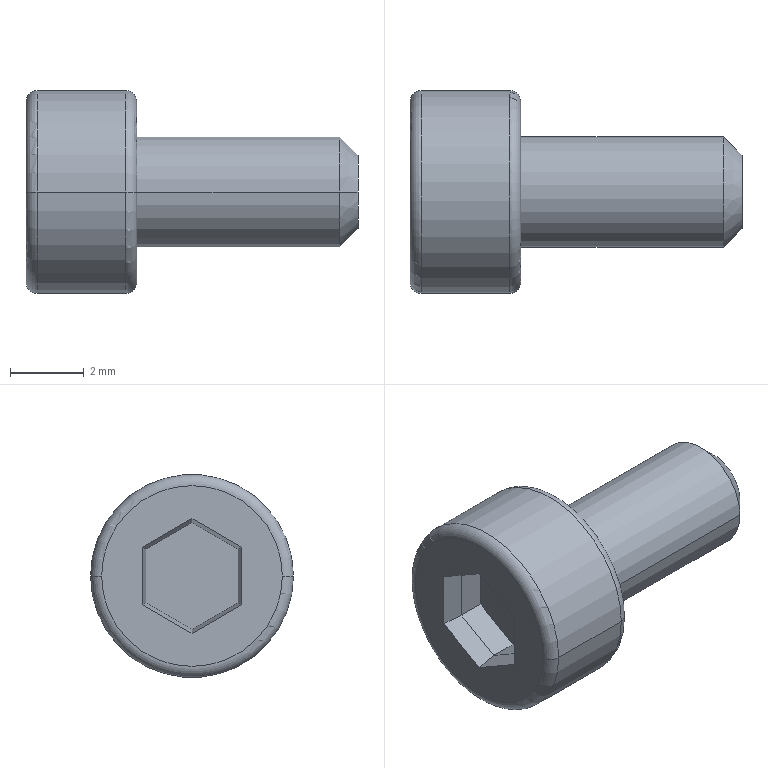Part | SolidWorks | features Chamfer 2, Fillet 1, ICE 1, Revolution 1 | 1 solid | 26 faces | box 9 x 5.5 x 5.5 mm | volume 104.699 mm3 | plane 16 | torus 4 | cylinder 4 | cone 2 | commonest cylinder face diameters 3 x2 5.5 x2
STEP:
#1=CARTESIAN_POINT('',(9.,1.,0.));
#2=VERTEX_POINT('',#1);
#3=CARTESIAN_POINT('',(9.,-1.,0.));
#4=VERTEX_POINT('',#3);
#5=CARTESIAN_POINT('',(9.,0.,0.));
#6=DIRECTION('',(1.,0.,0.));
#7=DIRECTION('',(0.,-1.,0.));
#8=AXIS2_PLACEMENT_3D('',#5,#6,#7);
#9=CIRCLE('',#8,1.);
#10=EDGE_CURVE('',#2,#4,#9,.T.);
#11=ORIENTED_EDGE('',*,*,#10,.F.);
#12=CARTESIAN_POINT('',(8.5,1.5,0.));
#13=VERTEX_POINT('',#12);
#14=CARTESIAN_POINT('',(8.5,1.5,0.));
#15=DIRECTION('',(-0.7071,0.7071,0.));
#16=VECTOR('',#15,1000.);
#17=LINE('',#14,#16);
#18=EDGE_CURVE('',#2,#13,#17,.T.);
#19=ORIENTED_EDGE('',*,*,#18,.T.);
#20=CARTESIAN_POINT('',(8.5,-1.5,0.));
#21=VERTEX_POINT('',#20);
#22=CARTESIAN_POINT('',(8.5,0.,0.));
#23=DIRECTION('',(-1.,0.,0.));
#24=DIRECTION('',(0.,-1.,0.));
#25=AXIS2_PLACEMENT_3D('',#22,#23,#24);
#26=CIRCLE('',#25,1.5);
#27=EDGE_CURVE('',#21,#13,#26,.T.);
#28=ORIENTED_EDGE('',*,*,#27,.F.);
#29=CARTESIAN_POINT('',(8.5,-1.5,0.));
#30=DIRECTION('',(-0.7071,-0.7071,0.));
#31=VECTOR('',#30,1000.);
#32=LINE('',#29,#31);
#33=EDGE_CURVE('',#4,#21,#32,.T.);
#34=ORIENTED_EDGE('',*,*,#33,.F.);
#35=EDGE_LOOP('',(#11,#19,#28,#34));
#36=FACE_OUTER_BOUND('',#35,.T.);
#37=CARTESIAN_POINT('',(8.5,0.,0.));
#38=DIRECTION('',(-1.,0.,0.));
#39=DIRECTION('',(0.,-1.,0.));
#40=AXIS2_PLACEMENT_3D('',#37,#38,#39);
#41=CONICAL_SURFACE('',#40,1.5,0.7854);
#42=ADVANCED_FACE('',(#36),#41,.T.);
#43=CARTESIAN_POINT('',(0.,-2.45,0.));
#44=VERTEX_POINT('',#43);
#45=CARTESIAN_POINT('',(0.,2.45,0.));
#46=VERTEX_POINT('',#45);
#47=CARTESIAN_POINT('',(0.,0.,0.));
#48=DIRECTION('',(-1.,0.,0.));
#49=DIRECTION('',(0.,1.,0.));
#50=AXIS2_PLACEMENT_3D('',#47,#48,#49);
#51=CIRCLE('',#50,2.45);
#52=EDGE_CURVE('',#44,#46,#51,.T.);
#53=ORIENTED_EDGE('',*,*,#52,.F.);
#54=CARTESIAN_POINT('',(0.3,-2.75,0.));
#55=VERTEX_POINT('',#54);
#56=CARTESIAN_POINT('',(0.3,-2.45,0.));
#57=DIRECTION('',(0.,0.,1.));
#58=DIRECTION('',(0.,-1.,0.));
#59=AXIS2_PLACEMENT_3D('',#56,#57,#58);
#60=CIRCLE('',#59,0.3);
#61=EDGE_CURVE('',#44,#55,#60,.T.);
#62=ORIENTED_EDGE('',*,*,#61,.T.);
#63=CARTESIAN_POINT('',(0.3,2.75,0.));
#64=VERTEX_POINT('',#63);
#65=CARTESIAN_POINT('',(0.3,0.,0.));
#66=DIRECTION('',(1.,0.,0.));
#67=DIRECTION('',(0.,1.,0.));
#68=AXIS2_PLACEMENT_3D('',#65,#66,#67);
#69=CIRCLE('',#68,2.75);
#70=EDGE_CURVE('',#64,#55,#69,.T.);
#71=ORIENTED_EDGE('',*,*,#70,.F.);
#72=CARTESIAN_POINT('',(0.3,2.45,0.));
#73=DIRECTION('',(0.,0.,-1.));
#74=DIRECTION('',(-1.,0.,0.));
#75=AXIS2_PLACEMENT_3D('',#72,#73,#74);
#76=CIRCLE('',#75,0.3);
#77=EDGE_CURVE('',#46,#64,#76,.T.);
#78=ORIENTED_EDGE('',*,*,#77,.F.);
#79=EDGE_LOOP('',(#53,#62,#71,#78));
#80=FACE_OUTER_BOUND('',#79,.T.);
#81=CARTESIAN_POINT('',(0.3,0.,0.));
#82=DIRECTION('',(1.,0.,0.));
#83=DIRECTION('',(0.,1.,0.));
#84=AXIS2_PLACEMENT_3D('',#81,#82,#83);
#85=TOROIDAL_SURFACE('',#84,2.45,0.3);
#86=ADVANCED_FACE('',(#80),#85,.T.);
#87=CARTESIAN_POINT('',(3.,2.45,0.));
#88=VERTEX_POINT('',#87);
#89=CARTESIAN_POINT('',(3.,-2.45,0.));
#90=VERTEX_POINT('',#89);
#91=CARTESIAN_POINT('',(3.,0.,0.));
#92=DIRECTION('',(1.,0.,0.));
#93=DIRECTION('',(0.,-1.,0.));
#94=AXIS2_PLACEMENT_3D('',#91,#92,#93);
#95=CIRCLE('',#94,2.45);
#96=EDGE_CURVE('',#88,#90,#95,.T.);
#97=ORIENTED_EDGE('',*,*,#96,.F.);
#98=CARTESIAN_POINT('',(2.7,2.75,0.));
#99=VERTEX_POINT('',#98);
#100=CARTESIAN_POINT('',(2.7,2.45,0.));
#101=DIRECTION('',(0.,0.,1.));
#102=DIRECTION('',(0.,-1.,0.));
#103=AXIS2_PLACEMENT_3D('',#100,#101,#102);
#104=CIRCLE('',#103,0.3);
#105=EDGE_CURVE('',#88,#99,#104,.T.);
#106=ORIENTED_EDGE('',*,*,#105,.T.);
#107=CARTESIAN_POINT('',(2.7,-2.75,0.));
#108=VERTEX_POINT('',#107);
#109=CARTESIAN_POINT('',(2.7,0.,0.));
#110=DIRECTION('',(-1.,0.,0.));
#111=DIRECTION('',(0.,-1.,0.));
#112=AXIS2_PLACEMENT_3D('',#109,#110,#111);
#113=CIRCLE('',#112,2.75);
#114=EDGE_CURVE('',#108,#99,#113,.T.);
#115=ORIENTED_EDGE('',*,*,#114,.F.);
#116=CARTESIAN_POINT('',(2.7,-2.45,0.));
#117=DIRECTION('',(0.,0.,-1.));
#118=DIRECTION('',(-1.,0.,0.));
#119=AXIS2_PLACEMENT_3D('',#116,#117,#118);
#120=CIRCLE('',#119,0.3);
#121=EDGE_CURVE('',#90,#108,#120,.T.);
#122=ORIENTED_EDGE('',*,*,#121,.F.);
#123=EDGE_LOOP('',(#97,#106,#115,#122));
#124=FACE_OUTER_BOUND('',#123,.T.);
#125=CARTESIAN_POINT('',(2.7,0.,0.));
#126=DIRECTION('',(-1.,0.,0.));
#127=DIRECTION('',(0.,-1.,0.));
#128=AXIS2_PLACEMENT_3D('',#125,#126,#127);
#129=TOROIDAL_SURFACE('',#128,2.45,0.3);
#130=ADVANCED_FACE('',(#124),#129,.T.);
#131=ORIENTED_EDGE('',*,*,#27,.T.);
#132=CARTESIAN_POINT('',(3.,1.5,0.));
#133=VERTEX_POINT('',#132);
#134=CARTESIAN_POINT('',(-4.709,1.5,0.));
#135=DIRECTION('',(-1.,0.,0.));
#136=VECTOR('',#135,1000.);
#137=LINE('',#134,#136);
#138=EDGE_CURVE('',#13,#133,#137,.T.);
#139=ORIENTED_EDGE('',*,*,#138,.T.);
#140=CARTESIAN_POINT('',(3.,-1.5,0.));
#141=VERTEX_POINT('',#140);
#142=CARTESIAN_POINT('',(3.,0.,0.));
#143=DIRECTION('',(-1.,0.,0.));
#144=DIRECTION('',(0.,-1.,0.));
#145=AXIS2_PLACEMENT_3D('',#142,#143,#144);
#146=CIRCLE('',#145,1.5);
#147=EDGE_CURVE('',#141,#133,#146,.T.);
#148=ORIENTED_EDGE('',*,*,#147,.F.);
#149=CARTESIAN_POINT('',(-4.709,-1.5,0.));
#150=DIRECTION('',(-1.,0.,0.));
#151=VECTOR('',#150,1000.);
#152=LINE('',#149,#151);
#153=EDGE_CURVE('',#21,#141,#152,.T.);
#154=ORIENTED_EDGE('',*,*,#153,.F.);
#155=EDGE_LOOP('',(#131,#139,#148,#154));
#156=FACE_OUTER_BOUND('',#155,.T.);
#157=CARTESIAN_POINT('',(-4.709,0.,0.));
#158=DIRECTION('',(-1.,0.,0.));
#159=DIRECTION('',(0.,-1.,0.));
#160=AXIS2_PLACEMENT_3D('',#157,#158,#159);
#161=CYLINDRICAL_SURFACE('',#160,1.5);
#162=ADVANCED_FACE('',(#156),#161,.T.);
#163=ORIENTED_EDGE('',*,*,#114,.T.);
#164=CARTESIAN_POINT('',(-4.709,2.75,0.));
#165=DIRECTION('',(-1.,0.,0.));
#166=VECTOR('',#165,1000.);
#167=LINE('',#164,#166);
#168=EDGE_CURVE('',#99,#64,#167,.T.);
#169=ORIENTED_EDGE('',*,*,#168,.T.);
#170=ORIENTED_EDGE('',*,*,#70,.T.);
#171=CARTESIAN_POINT('',(-4.709,-2.75,0.));
#172=DIRECTION('',(-1.,0.,0.));
#173=VECTOR('',#172,1000.);
#174=LINE('',#171,#173);
#175=EDGE_CURVE('',#108,#55,#174,.T.);
#176=ORIENTED_EDGE('',*,*,#175,.F.);
#177=EDGE_LOOP('',(#163,#169,#170,#176));
#178=FACE_OUTER_BOUND('',#177,.T.);
#179=CARTESIAN_POINT('',(-4.709,0.,0.));
#180=DIRECTION('',(-1.,0.,0.));
#181=DIRECTION('',(0.,-1.,0.));
#182=AXIS2_PLACEMENT_3D('',#179,#180,#181);
#183=CYLINDRICAL_SURFACE('',#182,2.75);
#184=ADVANCED_FACE('',(#178),#183,.T.);
#185=CARTESIAN_POINT('',(0.,-1.35,0.7794));
#186=VERTEX_POINT('',#185);
#187=CARTESIAN_POINT('',(0.,-1.35,-0.7794));
#188=VERTEX_POINT('',#187);
#189=CARTESIAN_POINT('',(0.,-1.35,0.));
#190=DIRECTION('',(0.,0.,-1.));
#191=VECTOR('',#190,1000.);
#192=LINE('',#189,#191);
#193=EDGE_CURVE('',#186,#188,#192,.T.);
#194=ORIENTED_EDGE('',*,*,#193,.T.);
#195=CARTESIAN_POINT('',(0.,0.,-1.559));
#196=VERTEX_POINT('',#195);
#197=CARTESIAN_POINT('',(0.,-0.675,-1.169));
#198=DIRECTION('',(0.,0.866,-0.5));
#199=VECTOR('',#198,1000.);
#200=LINE('',#197,#199);
#201=EDGE_CURVE('',#188,#196,#200,.T.);
#202=ORIENTED_EDGE('',*,*,#201,.T.);
#203=CARTESIAN_POINT('',(0.,1.35,-0.7794));
#204=VERTEX_POINT('',#203);
#205=CARTESIAN_POINT('',(0.,0.675,-1.169));
#206=DIRECTION('',(0.,0.866,0.5));
#207=VECTOR('',#206,1000.);
#208=LINE('',#205,#207);
#209=EDGE_CURVE('',#196,#204,#208,.T.);
#210=ORIENTED_EDGE('',*,*,#209,.T.);
#211=CARTESIAN_POINT('',(0.,1.35,0.7794));
#212=VERTEX_POINT('',#211);
#213=CARTESIAN_POINT('',(0.,1.35,0.));
#214=DIRECTION('',(0.,0.,1.));
#215=VECTOR('',#214,1000.);
#216=LINE('',#213,#215);
#217=EDGE_CURVE('',#204,#212,#216,.T.);
#218=ORIENTED_EDGE('',*,*,#217,.T.);
#219=CARTESIAN_POINT('',(0.,0.,1.559));
#220=VERTEX_POINT('',#219);
#221=CARTESIAN_POINT('',(0.,0.675,1.169));
#222=DIRECTION('',(0.,-0.866,0.5));
#223=VECTOR('',#222,1000.);
#224=LINE('',#221,#223);
#225=EDGE_CURVE('',#212,#220,#224,.T.);
#226=ORIENTED_EDGE('',*,*,#225,.T.);
#227=CARTESIAN_POINT('',(0.,-0.675,1.169));
#228=DIRECTION('',(0.,-0.866,-0.5));
#229=VECTOR('',#228,1000.);
#230=LINE('',#227,#229);
#231=EDGE_CURVE('',#220,#186,#230,.T.);
#232=ORIENTED_EDGE('',*,*,#231,.T.);
#233=EDGE_LOOP('',(#194,#202,#210,#218,#226,#232));
#234=FACE_BOUND('',#233,.T.);
#235=CARTESIAN_POINT('',(0.,0.,0.));
#236=DIRECTION('',(-1.,0.,0.));
#237=DIRECTION('',(0.,1.,0.));
#238=AXIS2_PLACEMENT_3D('',#235,#236,#237);
#239=CIRCLE('',#238,2.45);
#240=EDGE_CURVE('',#46,#44,#239,.T.);
#241=ORIENTED_EDGE('',*,*,#240,.T.);
#242=ORIENTED_EDGE('',*,*,#52,.T.);
#243=EDGE_LOOP('',(#241,#242));
#244=FACE_OUTER_BOUND('',#243,.T.);
#245=CARTESIAN_POINT('',(0.,0.,0.));
#246=DIRECTION('',(1.,0.,0.));
#247=DIRECTION('',(0.,1.,0.));
#248=AXIS2_PLACEMENT_3D('',#245,#246,#247);
#249=PLANE('',#248);
#250=ADVANCED_FACE('',(#234,#244),#249,.F.);
#251=ORIENTED_EDGE('',*,*,#168,.F.);
#252=CARTESIAN_POINT('',(2.7,0.,0.));
#253=DIRECTION('',(-1.,0.,0.));
#254=DIRECTION('',(0.,-1.,0.));
#255=AXIS2_PLACEMENT_3D('',#252,#253,#254);
#256=CIRCLE('',#255,2.75);
#257=EDGE_CURVE('',#99,#108,#256,.T.);
#258=ORIENTED_EDGE('',*,*,#257,.T.);
#259=ORIENTED_EDGE('',*,*,#175,.T.);
#260=CARTESIAN_POINT('',(0.3,0.,0.));
#261=DIRECTION('',(1.,0.,0.));
#262=DIRECTION('',(0.,1.,0.));
#263=AXIS2_PLACEMENT_3D('',#260,#261,#262);
#264=CIRCLE('',#263,2.75);
#265=EDGE_CURVE('',#55,#64,#264,.T.);
#266=ORIENTED_EDGE('',*,*,#265,.T.);
#267=EDGE_LOOP('',(#251,#258,#259,#266));
#268=FACE_OUTER_BOUND('',#267,.T.);
#269=CARTESIAN_POINT('',(-4.709,0.,0.));
#270=DIRECTION('',(-1.,0.,0.));
#271=DIRECTION('',(0.,-1.,0.));
#272=AXIS2_PLACEMENT_3D('',#269,#270,#271);
#273=CYLINDRICAL_SURFACE('',#272,2.75);
#274=ADVANCED_FACE('',(#268),#273,.T.);
#275=CARTESIAN_POINT('',(3.,0.,0.));
#276=DIRECTION('',(1.,0.,0.));
#277=DIRECTION('',(0.,-1.,0.));
#278=AXIS2_PLACEMENT_3D('',#275,#276,#277);
#279=CIRCLE('',#278,2.45);
#280=EDGE_CURVE('',#90,#88,#279,.T.);
#281=ORIENTED_EDGE('',*,*,#280,.T.);
#282=ORIENTED_EDGE('',*,*,#96,.T.);
#283=EDGE_LOOP('',(#281,#282));
#284=FACE_OUTER_BOUND('',#283,.T.);
#285=ORIENTED_EDGE('',*,*,#147,.T.);
#286=CARTESIAN_POINT('',(3.,0.,0.));
#287=DIRECTION('',(-1.,0.,0.));
#288=DIRECTION('',(0.,-1.,0.));
#289=AXIS2_PLACEMENT_3D('',#286,#287,#288);
#290=CIRCLE('',#289,1.5);
#291=EDGE_CURVE('',#133,#141,#290,.T.);
#292=ORIENTED_EDGE('',*,*,#291,.T.);
#293=EDGE_LOOP('',(#285,#292));
#294=FACE_BOUND('',#293,.T.);
#295=CARTESIAN_POINT('',(3.,2.75,0.));
#296=DIRECTION('',(-1.,0.,0.));
#297=DIRECTION('',(0.,-1.,0.));
#298=AXIS2_PLACEMENT_3D('',#295,#296,#297);
#299=PLANE('',#298);
#300=ADVANCED_FACE('',(#284,#294),#299,.F.);
#301=ORIENTED_EDGE('',*,*,#138,.F.);
#302=CARTESIAN_POINT('',(8.5,0.,0.));
#303=DIRECTION('',(-1.,0.,0.));
#304=DIRECTION('',(0.,-1.,0.));
#305=AXIS2_PLACEMENT_3D('',#302,#303,#304);
#306=CIRCLE('',#305,1.5);
#307=EDGE_CURVE('',#13,#21,#306,.T.);
#308=ORIENTED_EDGE('',*,*,#307,.T.);
#309=ORIENTED_EDGE('',*,*,#153,.T.);
#310=ORIENTED_EDGE('',*,*,#291,.F.);
#311=EDGE_LOOP('',(#301,#308,#309,#310));
#312=FACE_OUTER_BOUND('',#311,.T.);
#313=CARTESIAN_POINT('',(-4.709,0.,0.));
#314=DIRECTION('',(-1.,0.,0.));
#315=DIRECTION('',(0.,-1.,0.));
#316=AXIS2_PLACEMENT_3D('',#313,#314,#315);
#317=CYLINDRICAL_SURFACE('',#316,1.5);
#318=ADVANCED_FACE('',(#312),#317,.T.);
#319=CARTESIAN_POINT('',(9.,0.,0.));
#320=DIRECTION('',(1.,0.,0.));
#321=DIRECTION('',(0.,-1.,0.));
#322=AXIS2_PLACEMENT_3D('',#319,#320,#321);
#323=CIRCLE('',#322,1.);
#324=EDGE_CURVE('',#4,#2,#323,.T.);
#325=ORIENTED_EDGE('',*,*,#324,.T.);
#326=ORIENTED_EDGE('',*,*,#10,.T.);
#327=EDGE_LOOP('',(#325,#326));
#328=FACE_OUTER_BOUND('',#327,.T.);
#329=CARTESIAN_POINT('',(9.,1.5,0.));
#330=DIRECTION('',(-1.,0.,0.));
#331=DIRECTION('',(0.,-1.,0.));
#332=AXIS2_PLACEMENT_3D('',#329,#330,#331);
#333=PLANE('',#332);
#334=ADVANCED_FACE('',(#328),#333,.F.);
#335=CARTESIAN_POINT('',(1.3,1.25,-0.7217));
#336=VERTEX_POINT('',#335);
#337=CARTESIAN_POINT('',(0.5671,1.25,-0.7217));
#338=VERTEX_POINT('',#337);
#339=CARTESIAN_POINT('',(1.3,1.25,-0.7217));
#340=DIRECTION('',(-1.,0.,0.));
#341=VECTOR('',#340,1000.);
#342=LINE('',#339,#341);
#343=EDGE_CURVE('',#336,#338,#342,.T.);
#344=ORIENTED_EDGE('',*,*,#343,.T.);
#345=CARTESIAN_POINT('',(0.5671,0.,-1.443));
#346=VERTEX_POINT('',#345);
#347=CARTESIAN_POINT('',(0.5671,1.25,-0.7217));
#348=DIRECTION('',(0.,-0.866,-0.5));
#349=VECTOR('',#348,1000.);
#350=LINE('',#347,#349);
#351=EDGE_CURVE('',#338,#346,#350,.T.);
#352=ORIENTED_EDGE('',*,*,#351,.T.);
#353=CARTESIAN_POINT('',(1.3,0.,-1.443));
#354=VERTEX_POINT('',#353);
#355=CARTESIAN_POINT('',(1.3,0.,-1.443));
#356=DIRECTION('',(-1.,0.,0.));
#357=VECTOR('',#356,1000.);
#358=LINE('',#355,#357);
#359=EDGE_CURVE('',#354,#346,#358,.T.);
#360=ORIENTED_EDGE('',*,*,#359,.F.);
#361=CARTESIAN_POINT('',(1.3,1.25,-0.7217));
#362=DIRECTION('',(0.,-0.866,-0.5));
#363=VECTOR('',#362,1000.);
#364=LINE('',#361,#363);
#365=EDGE_CURVE('',#336,#354,#364,.T.);
#366=ORIENTED_EDGE('',*,*,#365,.F.);
#367=EDGE_LOOP('',(#344,#352,#360,#366));
#368=FACE_OUTER_BOUND('',#367,.T.);
#369=CARTESIAN_POINT('',(1.3,1.25,-0.7217));
#370=DIRECTION('',(0.,0.5,-0.866));
#371=DIRECTION('',(0.,0.866,0.5));
#372=AXIS2_PLACEMENT_3D('',#369,#370,#371);
#373=PLANE('',#372);
#374=ADVANCED_FACE('',(#368),#373,.F.);
#375=CARTESIAN_POINT('',(1.3,1.25,0.7217));
#376=VERTEX_POINT('',#375);
#377=CARTESIAN_POINT('',(0.5671,1.25,0.7217));
#378=VERTEX_POINT('',#377);
#379=CARTESIAN_POINT('',(1.3,1.25,0.7217));
#380=DIRECTION('',(-1.,0.,0.));
#381=VECTOR('',#380,1000.);
#382=LINE('',#379,#381);
#383=EDGE_CURVE('',#376,#378,#382,.T.);
#384=ORIENTED_EDGE('',*,*,#383,.T.);
#385=CARTESIAN_POINT('',(0.5671,1.25,0.7217));
#386=DIRECTION('',(0.,0.,-1.));
#387=VECTOR('',#386,1000.);
#388=LINE('',#385,#387);
#389=EDGE_CURVE('',#378,#338,#388,.T.);
#390=ORIENTED_EDGE('',*,*,#389,.T.);
#391=ORIENTED_EDGE('',*,*,#343,.F.);
#392=CARTESIAN_POINT('',(1.3,1.25,0.7217));
#393=DIRECTION('',(0.,0.,-1.));
#394=VECTOR('',#393,1000.);
#395=LINE('',#392,#394);
#396=EDGE_CURVE('',#376,#336,#395,.T.);
#397=ORIENTED_EDGE('',*,*,#396,.F.);
#398=EDGE_LOOP('',(#384,#390,#391,#397));
#399=FACE_OUTER_BOUND('',#398,.T.);
#400=CARTESIAN_POINT('',(1.3,1.25,0.7217));
#401=DIRECTION('',(0.,1.,0.));
#402=DIRECTION('',(0.,0.,1.));
#403=AXIS2_PLACEMENT_3D('',#400,#401,#402);
#404=PLANE('',#403);
#405=ADVANCED_FACE('',(#399),#404,.F.);
#406=CARTESIAN_POINT('',(1.3,0.,1.443));
#407=VERTEX_POINT('',#406);
#408=CARTESIAN_POINT('',(0.5671,0.,1.443));
#409=VERTEX_POINT('',#408);
#410=CARTESIAN_POINT('',(1.3,0.,1.443));
#411=DIRECTION('',(-1.,0.,0.));
#412=VECTOR('',#411,1000.);
#413=LINE('',#410,#412);
#414=EDGE_CURVE('',#407,#409,#413,.T.);
#415=ORIENTED_EDGE('',*,*,#414,.T.);
#416=CARTESIAN_POINT('',(0.5671,0.,1.443));
#417=DIRECTION('',(0.,0.866,-0.5));
#418=VECTOR('',#417,1000.);
#419=LINE('',#416,#418);
#420=EDGE_CURVE('',#409,#378,#419,.T.);
#421=ORIENTED_EDGE('',*,*,#420,.T.);
#422=ORIENTED_EDGE('',*,*,#383,.F.);
#423=CARTESIAN_POINT('',(1.3,0.,1.443));
#424=DIRECTION('',(0.,0.866,-0.5));
#425=VECTOR('',#424,1000.);
#426=LINE('',#423,#425);
#427=EDGE_CURVE('',#407,#376,#426,.T.);
#428=ORIENTED_EDGE('',*,*,#427,.F.);
#429=EDGE_LOOP('',(#415,#421,#422,#428));
#430=FACE_OUTER_BOUND('',#429,.T.);
#431=CARTESIAN_POINT('',(1.3,0.,1.443));
#432=DIRECTION('',(0.,0.5,0.866));
#433=DIRECTION('',(0.,-0.866,0.5));
#434=AXIS2_PLACEMENT_3D('',#431,#432,#433);
#435=PLANE('',#434);
#436=ADVANCED_FACE('',(#430),#435,.F.);
#437=CARTESIAN_POINT('',(1.3,-1.25,0.7217));
#438=VERTEX_POINT('',#437);
#439=CARTESIAN_POINT('',(0.5671,-1.25,0.7217));
#440=VERTEX_POINT('',#439);
#441=CARTESIAN_POINT('',(1.3,-1.25,0.7217));
#442=DIRECTION('',(-1.,0.,0.));
#443=VECTOR('',#442,1000.);
#444=LINE('',#441,#443);
#445=EDGE_CURVE('',#438,#440,#444,.T.);
#446=ORIENTED_EDGE('',*,*,#445,.T.);
#447=CARTESIAN_POINT('',(0.5671,-1.25,0.7217));
#448=DIRECTION('',(0.,0.866,0.5));
#449=VECTOR('',#448,1000.);
#450=LINE('',#447,#449);
#451=EDGE_CURVE('',#440,#409,#450,.T.);
#452=ORIENTED_EDGE('',*,*,#451,.T.);
#453=ORIENTED_EDGE('',*,*,#414,.F.);
#454=CARTESIAN_POINT('',(1.3,-1.25,0.7217));
#455=DIRECTION('',(0.,0.866,0.5));
#456=VECTOR('',#455,1000.);
#457=LINE('',#454,#456);
#458=EDGE_CURVE('',#438,#407,#457,.T.);
#459=ORIENTED_EDGE('',*,*,#458,.F.);
#460=EDGE_LOOP('',(#446,#452,#453,#459));
#461=FACE_OUTER_BOUND('',#460,.T.);
#462=CARTESIAN_POINT('',(1.3,-1.25,0.7217));
#463=DIRECTION('',(0.,-0.5,0.866));
#464=DIRECTION('',(0.,-0.866,-0.5));
#465=AXIS2_PLACEMENT_3D('',#462,#463,#464);
#466=PLANE('',#465);
#467=ADVANCED_FACE('',(#461),#466,.F.);
#468=CARTESIAN_POINT('',(1.3,-1.25,-0.7217));
#469=VERTEX_POINT('',#468);
#470=CARTESIAN_POINT('',(0.5671,-1.25,-0.7217));
#471=VERTEX_POINT('',#470);
#472=CARTESIAN_POINT('',(1.3,-1.25,-0.7217));
#473=DIRECTION('',(-1.,0.,0.));
#474=VECTOR('',#473,1000.);
#475=LINE('',#472,#474);
#476=EDGE_CURVE('',#469,#471,#475,.T.);
#477=ORIENTED_EDGE('',*,*,#476,.T.);
#478=CARTESIAN_POINT('',(0.5671,-1.25,-0.7217));
#479=DIRECTION('',(0.,0.,1.));
#480=VECTOR('',#479,1000.);
#481=LINE('',#478,#480);
#482=EDGE_CURVE('',#471,#440,#481,.T.);
#483=ORIENTED_EDGE('',*,*,#482,.T.);
#484=ORIENTED_EDGE('',*,*,#445,.F.);
#485=CARTESIAN_POINT('',(1.3,-1.25,-0.7217));
#486=DIRECTION('',(0.,0.,1.));
#487=VECTOR('',#486,1000.);
#488=LINE('',#485,#487);
#489=EDGE_CURVE('',#469,#438,#488,.T.);
#490=ORIENTED_EDGE('',*,*,#489,.F.);
#491=EDGE_LOOP('',(#477,#483,#484,#490));
#492=FACE_OUTER_BOUND('',#491,.T.);
#493=CARTESIAN_POINT('',(1.3,-1.25,-0.7217));
#494=DIRECTION('',(0.,-1.,0.));
#495=DIRECTION('',(0.,0.,-1.));
#496=AXIS2_PLACEMENT_3D('',#493,#494,#495);
#497=PLANE('',#496);
#498=ADVANCED_FACE('',(#492),#497,.F.);
#499=ORIENTED_EDGE('',*,*,#359,.T.);
#500=CARTESIAN_POINT('',(0.5671,0.,-1.443));
#501=DIRECTION('',(0.,-0.866,0.5));
#502=VECTOR('',#501,1000.);
#503=LINE('',#500,#502);
#504=EDGE_CURVE('',#346,#471,#503,.T.);
#505=ORIENTED_EDGE('',*,*,#504,.T.);
#506=ORIENTED_EDGE('',*,*,#476,.F.);
#507=CARTESIAN_POINT('',(1.3,0.,-1.443));
#508=DIRECTION('',(0.,-0.866,0.5));
#509=VECTOR('',#508,1000.);
#510=LINE('',#507,#509);
#511=EDGE_CURVE('',#354,#469,#510,.T.);
#512=ORIENTED_EDGE('',*,*,#511,.F.);
#513=EDGE_LOOP('',(#499,#505,#506,#512));
#514=FACE_OUTER_BOUND('',#513,.T.);
#515=CARTESIAN_POINT('',(1.3,0.,-1.443));
#516=DIRECTION('',(0.,-0.5,-0.866));
#517=DIRECTION('',(0.,0.866,-0.5));
#518=AXIS2_PLACEMENT_3D('',#515,#516,#517);
#519=PLANE('',#518);
#520=ADVANCED_FACE('',(#514),#519,.F.);
#521=ORIENTED_EDGE('',*,*,#365,.T.);
#522=ORIENTED_EDGE('',*,*,#511,.T.);
#523=ORIENTED_EDGE('',*,*,#489,.T.);
#524=ORIENTED_EDGE('',*,*,#458,.T.);
#525=ORIENTED_EDGE('',*,*,#427,.T.);
#526=ORIENTED_EDGE('',*,*,#396,.T.);
#527=EDGE_LOOP('',(#521,#522,#523,#524,#525,#526));
#528=FACE_OUTER_BOUND('',#527,.T.);
#529=CARTESIAN_POINT('',(1.3,0.,0.));
#530=DIRECTION('',(-1.,0.,0.));
#531=DIRECTION('',(0.,0.,1.));
#532=AXIS2_PLACEMENT_3D('',#529,#530,#531);
#533=PLANE('',#532);
#534=ADVANCED_FACE('',(#528),#533,.T.);
#535=ORIENTED_EDGE('',*,*,#105,.F.);
#536=ORIENTED_EDGE('',*,*,#280,.F.);
#537=ORIENTED_EDGE('',*,*,#121,.T.);
#538=ORIENTED_EDGE('',*,*,#257,.F.);
#539=EDGE_LOOP('',(#535,#536,#537,#538));
#540=FACE_OUTER_BOUND('',#539,.T.);
#541=CARTESIAN_POINT('',(2.7,0.,0.));
#542=DIRECTION('',(-1.,0.,0.));
#543=DIRECTION('',(0.,-1.,0.));
#544=AXIS2_PLACEMENT_3D('',#541,#542,#543);
#545=TOROIDAL_SURFACE('',#544,2.45,0.3);
#546=ADVANCED_FACE('',(#540),#545,.T.);
#547=ORIENTED_EDGE('',*,*,#61,.F.);
#548=ORIENTED_EDGE('',*,*,#240,.F.);
#549=ORIENTED_EDGE('',*,*,#77,.T.);
#550=ORIENTED_EDGE('',*,*,#265,.F.);
#551=EDGE_LOOP('',(#547,#548,#549,#550));
#552=FACE_OUTER_BOUND('',#551,.T.);
#553=CARTESIAN_POINT('',(0.3,0.,0.));
#554=DIRECTION('',(1.,0.,0.));
#555=DIRECTION('',(0.,1.,0.));
#556=AXIS2_PLACEMENT_3D('',#553,#554,#555);
#557=TOROIDAL_SURFACE('',#556,2.45,0.3);
#558=ADVANCED_FACE('',(#552),#557,.T.);
#559=CARTESIAN_POINT('',(0.7082,0.,1.415));
#560=DIRECTION('',(0.9799,0.,-0.1995));
#561=VECTOR('',#560,1000.);
#562=LINE('',#559,#561);
#563=EDGE_CURVE('',#220,#409,#562,.T.);
#564=ORIENTED_EDGE('',*,*,#563,.F.);
#565=ORIENTED_EDGE('',*,*,#225,.F.);
#566=CARTESIAN_POINT('',(0.7082,1.225,0.7073));
#567=DIRECTION('',(-0.9799,0.1728,0.09976));
#568=VECTOR('',#567,1000.);
#569=LINE('',#566,#568);
#570=EDGE_CURVE('',#378,#212,#569,.T.);
#571=ORIENTED_EDGE('',*,*,#570,.F.);
#572=ORIENTED_EDGE('',*,*,#420,.F.);
#573=EDGE_LOOP('',(#564,#565,#571,#572));
#574=FACE_OUTER_BOUND('',#573,.T.);
#575=CARTESIAN_POINT('',(0.5671,0.,1.443));
#576=DIRECTION('',(0.1736,0.4924,0.8529));
#577=DIRECTION('',(0.,0.866,-0.5));
#578=AXIS2_PLACEMENT_3D('',#575,#576,#577);
#579=PLANE('',#578);
#580=ADVANCED_FACE('',(#574),#579,.F.);
#581=ORIENTED_EDGE('',*,*,#570,.T.);
#582=ORIENTED_EDGE('',*,*,#217,.F.);
#583=CARTESIAN_POINT('',(0.7082,1.225,-0.7073));
#584=DIRECTION('',(-0.9799,0.1728,-0.09976));
#585=VECTOR('',#584,1000.);
#586=LINE('',#583,#585);
#587=EDGE_CURVE('',#338,#204,#586,.T.);
#588=ORIENTED_EDGE('',*,*,#587,.F.);
#589=ORIENTED_EDGE('',*,*,#389,.F.);
#590=EDGE_LOOP('',(#581,#582,#588,#589));
#591=FACE_OUTER_BOUND('',#590,.T.);
#592=CARTESIAN_POINT('',(0.5671,1.25,0.7217));
#593=DIRECTION('',(0.1736,0.9848,0.));
#594=DIRECTION('',(0.,0.,-1.));
#595=AXIS2_PLACEMENT_3D('',#592,#593,#594);
#596=PLANE('',#595);
#597=ADVANCED_FACE('',(#591),#596,.F.);
#598=ORIENTED_EDGE('',*,*,#563,.T.);
#599=ORIENTED_EDGE('',*,*,#451,.F.);
#600=CARTESIAN_POINT('',(0.7082,-1.225,0.7073));
#601=DIRECTION('',(0.9799,0.1728,-0.09976));
#602=VECTOR('',#601,1000.);
#603=LINE('',#600,#602);
#604=EDGE_CURVE('',#186,#440,#603,.T.);
#605=ORIENTED_EDGE('',*,*,#604,.F.);
#606=ORIENTED_EDGE('',*,*,#231,.F.);
#607=EDGE_LOOP('',(#598,#599,#605,#606));
#608=FACE_OUTER_BOUND('',#607,.T.);
#609=CARTESIAN_POINT('',(0.5671,-1.25,0.7217));
#610=DIRECTION('',(0.1736,-0.4924,0.8529));
#611=DIRECTION('',(0.,0.866,0.5));
#612=AXIS2_PLACEMENT_3D('',#609,#610,#611);
#613=PLANE('',#612);
#614=ADVANCED_FACE('',(#608),#613,.F.);
#615=ORIENTED_EDGE('',*,*,#587,.T.);
#616=ORIENTED_EDGE('',*,*,#209,.F.);
#617=CARTESIAN_POINT('',(0.5671,0.,-1.443));
#618=DIRECTION('',(-0.9799,0.,-0.1995));
#619=VECTOR('',#618,1000.);
#620=LINE('',#617,#619);
#621=EDGE_CURVE('',#346,#196,#620,.T.);
#622=ORIENTED_EDGE('',*,*,#621,.F.);
#623=ORIENTED_EDGE('',*,*,#351,.F.);
#624=EDGE_LOOP('',(#615,#616,#622,#623));
#625=FACE_OUTER_BOUND('',#624,.T.);
#626=CARTESIAN_POINT('',(0.5671,1.25,-0.7217));
#627=DIRECTION('',(0.1736,0.4924,-0.8529));
#628=DIRECTION('',(0.,-0.866,-0.5));
#629=AXIS2_PLACEMENT_3D('',#626,#627,#628);
#630=PLANE('',#629);
#631=ADVANCED_FACE('',(#625),#630,.F.);
#632=ORIENTED_EDGE('',*,*,#604,.T.);
#633=ORIENTED_EDGE('',*,*,#482,.F.);
#634=CARTESIAN_POINT('',(0.7082,-1.225,-0.7073));
#635=DIRECTION('',(0.9799,0.1728,0.09976));
#636=VECTOR('',#635,1000.);
#637=LINE('',#634,#636);
#638=EDGE_CURVE('',#188,#471,#637,.T.);
#639=ORIENTED_EDGE('',*,*,#638,.F.);
#640=ORIENTED_EDGE('',*,*,#193,.F.);
#641=EDGE_LOOP('',(#632,#633,#639,#640));
#642=FACE_OUTER_BOUND('',#641,.T.);
#643=CARTESIAN_POINT('',(0.5671,-1.25,-0.7217));
#644=DIRECTION('',(0.1736,-0.9848,0.));
#645=DIRECTION('',(0.,0.,1.));
#646=AXIS2_PLACEMENT_3D('',#643,#644,#645);
#647=PLANE('',#646);
#648=ADVANCED_FACE('',(#642),#647,.F.);
#649=ORIENTED_EDGE('',*,*,#621,.T.);
#650=ORIENTED_EDGE('',*,*,#201,.F.);
#651=ORIENTED_EDGE('',*,*,#638,.T.);
#652=ORIENTED_EDGE('',*,*,#504,.F.);
#653=EDGE_LOOP('',(#649,#650,#651,#652));
#654=FACE_OUTER_BOUND('',#653,.T.);
#655=CARTESIAN_POINT('',(0.5671,0.,-1.443));
#656=DIRECTION('',(0.1736,-0.4924,-0.8529));
#657=DIRECTION('',(0.,-0.866,0.5));
#658=AXIS2_PLACEMENT_3D('',#655,#656,#657);
#659=PLANE('',#658);
#660=ADVANCED_FACE('',(#654),#659,.F.);
#661=ORIENTED_EDGE('',*,*,#18,.F.);
#662=ORIENTED_EDGE('',*,*,#324,.F.);
#663=ORIENTED_EDGE('',*,*,#33,.T.);
#664=ORIENTED_EDGE('',*,*,#307,.F.);
#665=EDGE_LOOP('',(#661,#662,#663,#664));
#666=FACE_OUTER_BOUND('',#665,.T.);
#667=CARTESIAN_POINT('',(8.5,0.,0.));
#668=DIRECTION('',(-1.,0.,0.));
#669=DIRECTION('',(0.,-1.,0.));
#670=AXIS2_PLACEMENT_3D('',#667,#668,#669);
#671=CONICAL_SURFACE('',#670,1.5,0.7854);
#672=ADVANCED_FACE('',(#666),#671,.T.);
#673=CLOSED_SHELL('',(#42,#86,#130,#162,#184,#250,#274,#300,#318,#334,#374,#405,#436,#467,#498,#520,#534,#546,#558,#580,#597,#614,#631,#648,#660,#672));
#674=MANIFOLD_SOLID_BREP('',#673);
#675=CARTESIAN_POINT('',(0.,0.,0.));
#676=DIRECTION('',(0.,0.,1.));
#677=DIRECTION('',(1.,0.,0.));
#678=AXIS2_PLACEMENT_3D('',#675,#676,#677);
#679=(LENGTH_UNIT()NAMED_UNIT(*)SI_UNIT(.MILLI.,.METRE.));
#680=UNCERTAINTY_MEASURE_WITH_UNIT(LENGTH_MEASURE(0.00001),#679,'','');
#681=(NAMED_UNIT(*)PLANE_ANGLE_UNIT()SI_UNIT($,.RADIAN.));
#682=(NAMED_UNIT(*)SI_UNIT($,.STERADIAN.)SOLID_ANGLE_UNIT());
#683=(GEOMETRIC_REPRESENTATION_CONTEXT(3)GLOBAL_UNCERTAINTY_ASSIGNED_CONTEXT((#680))GLOBAL_UNIT_ASSIGNED_CONTEXT((#679,#681,#682))REPRESENTATION_CONTEXT('',''));
#684=ADVANCED_BREP_SHAPE_REPRESENTATION('',(#674,#678),#683);